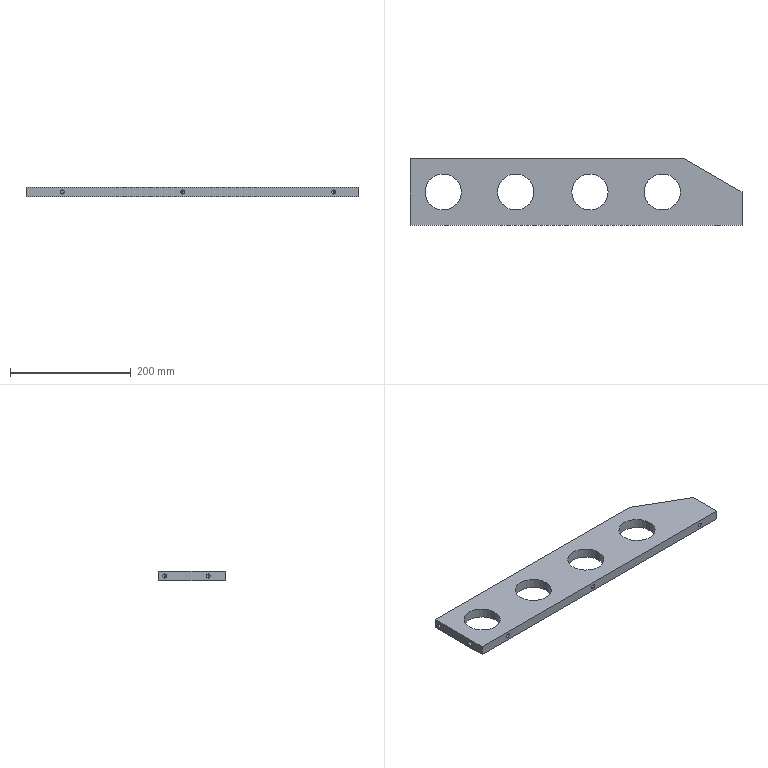Part | SolidWorks | features HoleWzd 4, ICE 4, LibraryFeature 2, Chamfer 1, Cut 1, Extrusion 1, Fillet 1 | 1 solid | 34 faces | box 550 x 110 x 16 mm | volume 740256 mm3 | cylinder 18 | cone 9 | plane 7 | commonest cylinder face diameters 6.75 x10 60 x8
STEP:
#1=CARTESIAN_POINT('',(-130.,0.,-8.));
#2=VERTEX_POINT('',#1);
#3=CARTESIAN_POINT('',(-70.,0.,-8.));
#4=VERTEX_POINT('',#3);
#5=CARTESIAN_POINT('',(-100.,0.,-8.));
#6=DIRECTION('',(0.,0.,1.));
#7=DIRECTION('',(1.,0.,0.));
#8=AXIS2_PLACEMENT_3D('',#5,#6,#7);
#9=CIRCLE('',#8,30.);
#10=EDGE_CURVE('',#2,#4,#9,.T.);
#11=ORIENTED_EDGE('',*,*,#10,.F.);
#12=CARTESIAN_POINT('',(-130.,0.,8.));
#13=VERTEX_POINT('',#12);
#14=CARTESIAN_POINT('',(-130.,0.,-8.));
#15=DIRECTION('',(0.,0.,1.));
#16=VECTOR('',#15,1000.);
#17=LINE('',#14,#16);
#18=EDGE_CURVE('',#2,#13,#17,.T.);
#19=ORIENTED_EDGE('',*,*,#18,.T.);
#20=CARTESIAN_POINT('',(-70.,0.,8.));
#21=VERTEX_POINT('',#20);
#22=CARTESIAN_POINT('',(-100.,0.,8.));
#23=DIRECTION('',(0.,0.,1.));
#24=DIRECTION('',(1.,0.,0.));
#25=AXIS2_PLACEMENT_3D('',#22,#23,#24);
#26=CIRCLE('',#25,30.);
#27=EDGE_CURVE('',#13,#21,#26,.T.);
#28=ORIENTED_EDGE('',*,*,#27,.T.);
#29=CARTESIAN_POINT('',(-70.,0.,-8.));
#30=DIRECTION('',(0.,0.,1.));
#31=VECTOR('',#30,1000.);
#32=LINE('',#29,#31);
#33=EDGE_CURVE('',#4,#21,#32,.T.);
#34=ORIENTED_EDGE('',*,*,#33,.F.);
#35=EDGE_LOOP('',(#11,#19,#28,#34));
#36=FACE_OUTER_BOUND('',#35,.T.);
#37=CARTESIAN_POINT('',(-100.,0.,-8.));
#38=DIRECTION('',(0.,0.,1.));
#39=DIRECTION('',(1.,0.,0.));
#40=AXIS2_PLACEMENT_3D('',#37,#38,#39);
#41=CYLINDRICAL_SURFACE('',#40,30.);
#42=ADVANCED_FACE('',(#36),#41,.F.);
#43=CARTESIAN_POINT('',(-6.962,0.,-8.));
#44=VERTEX_POINT('',#43);
#45=CARTESIAN_POINT('',(53.038,0.,-8.));
#46=VERTEX_POINT('',#45);
#47=CARTESIAN_POINT('',(23.038,0.,-8.));
#48=DIRECTION('',(0.,0.,1.));
#49=DIRECTION('',(-1.,0.,0.));
#50=AXIS2_PLACEMENT_3D('',#47,#48,#49);
#51=CIRCLE('',#50,30.);
#52=EDGE_CURVE('',#44,#46,#51,.T.);
#53=ORIENTED_EDGE('',*,*,#52,.F.);
#54=CARTESIAN_POINT('',(-6.962,0.,8.));
#55=VERTEX_POINT('',#54);
#56=CARTESIAN_POINT('',(-6.962,0.,-8.));
#57=DIRECTION('',(0.,0.,1.));
#58=VECTOR('',#57,1000.);
#59=LINE('',#56,#58);
#60=EDGE_CURVE('',#44,#55,#59,.T.);
#61=ORIENTED_EDGE('',*,*,#60,.T.);
#62=CARTESIAN_POINT('',(53.038,0.,8.));
#63=VERTEX_POINT('',#62);
#64=CARTESIAN_POINT('',(23.038,0.,8.));
#65=DIRECTION('',(0.,0.,1.));
#66=DIRECTION('',(-1.,0.,0.));
#67=AXIS2_PLACEMENT_3D('',#64,#65,#66);
#68=CIRCLE('',#67,30.);
#69=EDGE_CURVE('',#55,#63,#68,.T.);
#70=ORIENTED_EDGE('',*,*,#69,.T.);
#71=CARTESIAN_POINT('',(53.038,0.,-8.));
#72=DIRECTION('',(0.,0.,1.));
#73=VECTOR('',#72,1000.);
#74=LINE('',#71,#73);
#75=EDGE_CURVE('',#46,#63,#74,.T.);
#76=ORIENTED_EDGE('',*,*,#75,.F.);
#77=EDGE_LOOP('',(#53,#61,#70,#76));
#78=FACE_OUTER_BOUND('',#77,.T.);
#79=CARTESIAN_POINT('',(23.038,0.,-8.));
#80=DIRECTION('',(0.,0.,1.));
#81=DIRECTION('',(1.,0.,0.));
#82=AXIS2_PLACEMENT_3D('',#79,#80,#81);
#83=CYLINDRICAL_SURFACE('',#82,30.);
#84=ADVANCED_FACE('',(#78),#83,.F.);
#85=CARTESIAN_POINT('',(113.038,0.,-8.));
#86=VERTEX_POINT('',#85);
#87=CARTESIAN_POINT('',(173.038,0.,-8.));
#88=VERTEX_POINT('',#87);
#89=CARTESIAN_POINT('',(143.038,0.,-8.));
#90=DIRECTION('',(0.,0.,1.));
#91=DIRECTION('',(-1.,0.,0.));
#92=AXIS2_PLACEMENT_3D('',#89,#90,#91);
#93=CIRCLE('',#92,30.);
#94=EDGE_CURVE('',#86,#88,#93,.T.);
#95=ORIENTED_EDGE('',*,*,#94,.F.);
#96=CARTESIAN_POINT('',(113.038,0.,8.));
#97=VERTEX_POINT('',#96);
#98=CARTESIAN_POINT('',(113.038,0.,-8.));
#99=DIRECTION('',(0.,0.,1.));
#100=VECTOR('',#99,1000.);
#101=LINE('',#98,#100);
#102=EDGE_CURVE('',#86,#97,#101,.T.);
#103=ORIENTED_EDGE('',*,*,#102,.T.);
#104=CARTESIAN_POINT('',(173.038,0.,8.));
#105=VERTEX_POINT('',#104);
#106=CARTESIAN_POINT('',(143.038,0.,8.));
#107=DIRECTION('',(0.,0.,1.));
#108=DIRECTION('',(-1.,0.,0.));
#109=AXIS2_PLACEMENT_3D('',#106,#107,#108);
#110=CIRCLE('',#109,30.);
#111=EDGE_CURVE('',#97,#105,#110,.T.);
#112=ORIENTED_EDGE('',*,*,#111,.T.);
#113=CARTESIAN_POINT('',(173.038,0.,-8.));
#114=DIRECTION('',(0.,0.,1.));
#115=VECTOR('',#114,1000.);
#116=LINE('',#113,#115);
#117=EDGE_CURVE('',#88,#105,#116,.T.);
#118=ORIENTED_EDGE('',*,*,#117,.F.);
#119=EDGE_LOOP('',(#95,#103,#112,#118));
#120=FACE_OUTER_BOUND('',#119,.T.);
#121=CARTESIAN_POINT('',(143.038,0.,-8.));
#122=DIRECTION('',(0.,0.,1.));
#123=DIRECTION('',(1.,0.,0.));
#124=AXIS2_PLACEMENT_3D('',#121,#122,#123);
#125=CYLINDRICAL_SURFACE('',#124,30.);
#126=ADVANCED_FACE('',(#120),#125,.F.);
#127=CARTESIAN_POINT('',(-212.319,-29.,2.05));
#128=VERTEX_POINT('',#127);
#129=CARTESIAN_POINT('',(-212.319,-29.,-2.05));
#130=VERTEX_POINT('',#129);
#131=CARTESIAN_POINT('',(-212.319,-29.,2.05));
#132=CARTESIAN_POINT('',(-212.241,-28.979,1.891));
#133=CARTESIAN_POINT('',(-212.171,-28.961,1.727));
#134=CARTESIAN_POINT('',(-212.053,-28.928,1.395));
#135=CARTESIAN_POINT('',(-212.003,-28.915,1.226));
#136=CARTESIAN_POINT('',(-211.883,-28.881,0.711));
#137=CARTESIAN_POINT('',(-211.842,-28.869,0.352));
#138=CARTESIAN_POINT('',(-211.842,-28.87,-0.3557));
#139=CARTESIAN_POINT('',(-211.882,-28.881,-0.7066));
#140=CARTESIAN_POINT('',(-212.045,-28.926,-1.403));
#141=CARTESIAN_POINT('',(-212.164,-28.959,-1.734));
#142=CARTESIAN_POINT('',(-212.319,-29.,-2.05));
#143=B_SPLINE_CURVE_WITH_KNOTS('',3,(#131,#132,#133,#134,#135,#136,#137,#138,#139,#140,#141,#142),.UNSPECIFIED.,.F.,.F.,(4,2,2,2,2,4),(0.001429,0.001958,0.002488,0.003547,0.004606,0.005665),.UNSPECIFIED.);
#144=EDGE_CURVE('',#128,#130,#143,.T.);
#145=ORIENTED_EDGE('',*,*,#144,.F.);
#146=CARTESIAN_POINT('',(-215.,-29.58,3.375));
#147=VERTEX_POINT('',#146);
#148=CARTESIAN_POINT('',(-215.,-29.58,3.375));
#149=CARTESIAN_POINT('',(-214.739,-29.536,3.375));
#150=CARTESIAN_POINT('',(-214.483,-29.489,3.345));
#151=CARTESIAN_POINT('',(-213.983,-29.391,3.228));
#152=CARTESIAN_POINT('',(-213.736,-29.34,3.14));
#153=CARTESIAN_POINT('',(-213.276,-29.238,2.913));
#154=CARTESIAN_POINT('',(-213.06,-29.187,2.774));
#155=CARTESIAN_POINT('',(-212.658,-29.088,2.444));
#156=CARTESIAN_POINT('',(-212.478,-29.042,2.258));
#157=CARTESIAN_POINT('',(-212.319,-29.,2.05));
#158=B_SPLINE_CURVE_WITH_KNOTS('',3,(#148,#149,#150,#151,#152,#153,#154,#155,#156,#157),.UNSPECIFIED.,.F.,.F.,(4,2,2,2,4),(0.01373,0.01451,0.01529,0.01608,0.01686),.UNSPECIFIED.);
#159=EDGE_CURVE('',#147,#128,#158,.T.);
#160=ORIENTED_EDGE('',*,*,#159,.F.);
#161=CARTESIAN_POINT('',(-215.,-29.58,-3.375));
#162=VERTEX_POINT('',#161);
#163=CARTESIAN_POINT('',(-215.,-29.58,-3.375));
#164=CARTESIAN_POINT('',(-215.218,-29.617,-3.375));
#165=CARTESIAN_POINT('',(-215.44,-29.652,-3.353));
#166=CARTESIAN_POINT('',(-215.87,-29.715,-3.268));
#167=CARTESIAN_POINT('',(-216.079,-29.743,-3.205));
#168=CARTESIAN_POINT('',(-216.487,-29.794,-3.038));
#169=CARTESIAN_POINT('',(-216.685,-29.817,-2.933));
#170=CARTESIAN_POINT('',(-217.051,-29.855,-2.689));
#171=CARTESIAN_POINT('',(-217.222,-29.872,-2.55));
#172=CARTESIAN_POINT('',(-217.538,-29.899,-2.236));
#173=CARTESIAN_POINT('',(-217.679,-29.91,-2.064));
#174=CARTESIAN_POINT('',(-217.925,-29.928,-1.698));
#175=CARTESIAN_POINT('',(-218.031,-29.935,-1.501));
#176=CARTESIAN_POINT('',(-218.202,-29.946,-1.09));
#177=CARTESIAN_POINT('',(-218.266,-29.95,-0.8789));
#178=CARTESIAN_POINT('',(-218.353,-29.955,-0.4449));
#179=CARTESIAN_POINT('',(-218.375,-29.956,-0.2203));
#180=CARTESIAN_POINT('',(-218.375,-29.956,0.2219));
#181=CARTESIAN_POINT('',(-218.353,-29.955,0.4417));
#182=CARTESIAN_POINT('',(-218.266,-29.95,0.8784));
#183=CARTESIAN_POINT('',(-218.201,-29.946,1.092));
#184=CARTESIAN_POINT('',(-218.031,-29.935,1.5));
#185=CARTESIAN_POINT('',(-217.926,-29.928,1.696));
#186=CARTESIAN_POINT('',(-217.678,-29.91,2.066));
#187=CARTESIAN_POINT('',(-217.537,-29.899,2.236));
#188=CARTESIAN_POINT('',(-217.225,-29.872,2.548));
#189=CARTESIAN_POINT('',(-217.05,-29.855,2.69));
#190=CARTESIAN_POINT('',(-216.683,-29.817,2.934));
#191=CARTESIAN_POINT('',(-216.489,-29.795,3.037));
#192=CARTESIAN_POINT('',(-216.081,-29.744,3.205));
#193=CARTESIAN_POINT('',(-215.867,-29.715,3.269));
#194=CARTESIAN_POINT('',(-215.438,-29.652,3.354));
#195=CARTESIAN_POINT('',(-215.221,-29.618,3.375));
#196=CARTESIAN_POINT('',(-215.,-29.58,3.375));
#197=B_SPLINE_CURVE_WITH_KNOTS('',3,(#163,#164,#165,#166,#167,#168,#169,#170,#171,#172,#173,#174,#175,#176,#177,#178,#179,#180,#181,#182,#183,#184,#185,#186,#187,#188,#189,#190,#191,#192,#193,#194,#195,#196),.UNSPECIFIED.,.F.,.F.,(4,2,2,2,2,2,2,2,2,2,2,2,2,2,2,2,4),(0.003138,0.0038,0.004462,0.005124,0.005786,0.006447,0.007109,0.007771,0.008433,0.009095,0.009756,0.01042,0.01108,0.01174,0.0124,0.01307,0.01373),.UNSPECIFIED.);
#198=EDGE_CURVE('',#162,#147,#197,.T.);
#199=ORIENTED_EDGE('',*,*,#198,.F.);
#200=CARTESIAN_POINT('',(-212.319,-29.,-2.05));
#201=CARTESIAN_POINT('',(-212.478,-29.042,-2.258));
#202=CARTESIAN_POINT('',(-212.657,-29.088,-2.443));
#203=CARTESIAN_POINT('',(-213.055,-29.186,-2.77));
#204=CARTESIAN_POINT('',(-213.276,-29.238,-2.913));
#205=CARTESIAN_POINT('',(-213.736,-29.34,-3.14));
#206=CARTESIAN_POINT('',(-213.979,-29.391,-3.227));
#207=CARTESIAN_POINT('',(-214.486,-29.49,-3.346));
#208=CARTESIAN_POINT('',(-214.742,-29.537,-3.375));
#209=CARTESIAN_POINT('',(-215.,-29.58,-3.375));
#210=B_SPLINE_CURVE_WITH_KNOTS('',3,(#200,#201,#202,#203,#204,#205,#206,#207,#208,#209),.UNSPECIFIED.,.F.,.F.,(4,2,2,2,4),(0.,0.0007846,0.001569,0.002354,0.003138),.UNSPECIFIED.);
#211=EDGE_CURVE('',#130,#162,#210,.T.);
#212=ORIENTED_EDGE('',*,*,#211,.F.);
#213=EDGE_LOOP('',(#145,#160,#199,#212));
#214=FACE_BOUND('',#213,.T.);
#215=CARTESIAN_POINT('',(-250.,0.,-8.));
#216=VERTEX_POINT('',#215);
#217=CARTESIAN_POINT('',(-190.,0.,-8.));
#218=VERTEX_POINT('',#217);
#219=CARTESIAN_POINT('',(-220.,0.,-8.));
#220=DIRECTION('',(0.,0.,1.));
#221=DIRECTION('',(1.,0.,0.));
#222=AXIS2_PLACEMENT_3D('',#219,#220,#221);
#223=CIRCLE('',#222,30.);
#224=EDGE_CURVE('',#216,#218,#223,.T.);
#225=ORIENTED_EDGE('',*,*,#224,.F.);
#226=CARTESIAN_POINT('',(-250.,0.,8.));
#227=VERTEX_POINT('',#226);
#228=CARTESIAN_POINT('',(-250.,0.,-8.));
#229=DIRECTION('',(0.,0.,1.));
#230=VECTOR('',#229,1000.);
#231=LINE('',#228,#230);
#232=EDGE_CURVE('',#216,#227,#231,.T.);
#233=ORIENTED_EDGE('',*,*,#232,.T.);
#234=CARTESIAN_POINT('',(-190.,0.,8.));
#235=VERTEX_POINT('',#234);
#236=CARTESIAN_POINT('',(-220.,0.,8.));
#237=DIRECTION('',(0.,0.,1.));
#238=DIRECTION('',(1.,0.,0.));
#239=AXIS2_PLACEMENT_3D('',#236,#237,#238);
#240=CIRCLE('',#239,30.);
#241=EDGE_CURVE('',#227,#235,#240,.T.);
#242=ORIENTED_EDGE('',*,*,#241,.T.);
#243=CARTESIAN_POINT('',(-190.,0.,-8.));
#244=DIRECTION('',(0.,0.,1.));
#245=VECTOR('',#244,1000.);
#246=LINE('',#243,#245);
#247=EDGE_CURVE('',#218,#235,#246,.T.);
#248=ORIENTED_EDGE('',*,*,#247,.F.);
#249=EDGE_LOOP('',(#225,#233,#242,#248));
#250=FACE_OUTER_BOUND('',#249,.T.);
#251=CARTESIAN_POINT('',(-220.,0.,-8.));
#252=DIRECTION('',(0.,0.,1.));
#253=DIRECTION('',(1.,0.,0.));
#254=AXIS2_PLACEMENT_3D('',#251,#252,#253);
#255=CYLINDRICAL_SURFACE('',#254,30.);
#256=ADVANCED_FACE('',(#214,#250),#255,.F.);
#257=CARTESIAN_POINT('',(-244.972,-27.,0.));
#258=VERTEX_POINT('',#257);
#259=CARTESIAN_POINT('',(-247.,-27.,3.375));
#260=VERTEX_POINT('',#259);
#261=CARTESIAN_POINT('',(-247.,-27.,3.375));
#262=DIRECTION('',(-0.515,0.,0.8572));
#263=VECTOR('',#262,1000.);
#264=LINE('',#261,#263);
#265=EDGE_CURVE('',#258,#260,#264,.T.);
#266=ORIENTED_EDGE('',*,*,#265,.F.);
#267=CARTESIAN_POINT('',(-247.,-27.,-3.375));
#268=VERTEX_POINT('',#267);
#269=CARTESIAN_POINT('',(-247.,-27.,-3.375));
#270=DIRECTION('',(-0.515,0.,-0.8572));
#271=VECTOR('',#270,1000.);
#272=LINE('',#269,#271);
#273=EDGE_CURVE('',#258,#268,#272,.T.);
#274=ORIENTED_EDGE('',*,*,#273,.T.);
#275=CARTESIAN_POINT('',(-247.,-27.,0.));
#276=DIRECTION('',(-1.,0.,0.));
#277=DIRECTION('',(0.,0.,1.));
#278=AXIS2_PLACEMENT_3D('',#275,#276,#277);
#279=CIRCLE('',#278,3.375);
#280=EDGE_CURVE('',#268,#260,#279,.T.);
#281=ORIENTED_EDGE('',*,*,#280,.T.);
#282=EDGE_LOOP('',(#266,#274,#281));
#283=FACE_OUTER_BOUND('',#282,.T.);
#284=CARTESIAN_POINT('',(-247.,-27.,0.));
#285=DIRECTION('',(-1.,0.,0.));
#286=DIRECTION('',(0.,0.,1.));
#287=AXIS2_PLACEMENT_3D('',#284,#285,#286);
#288=CONICAL_SURFACE('',#287,3.375,1.03);
#289=ADVANCED_FACE('',(#283),#288,.F.);
#290=ORIENTED_EDGE('',*,*,#280,.F.);
#291=CARTESIAN_POINT('',(-275.,-27.,-3.375));
#292=VERTEX_POINT('',#291);
#293=CARTESIAN_POINT('',(-275.,-27.,-3.375));
#294=DIRECTION('',(-1.,0.,0.));
#295=VECTOR('',#294,1000.);
#296=LINE('',#293,#295);
#297=EDGE_CURVE('',#268,#292,#296,.T.);
#298=ORIENTED_EDGE('',*,*,#297,.T.);
#299=CARTESIAN_POINT('',(-275.,-27.,3.375));
#300=VERTEX_POINT('',#299);
#301=CARTESIAN_POINT('',(-275.,-27.,0.));
#302=DIRECTION('',(-1.,0.,0.));
#303=DIRECTION('',(0.,0.,1.));
#304=AXIS2_PLACEMENT_3D('',#301,#302,#303);
#305=CIRCLE('',#304,3.375);
#306=EDGE_CURVE('',#292,#300,#305,.T.);
#307=ORIENTED_EDGE('',*,*,#306,.T.);
#308=CARTESIAN_POINT('',(-275.,-27.,3.375));
#309=DIRECTION('',(-1.,0.,0.));
#310=VECTOR('',#309,1000.);
#311=LINE('',#308,#310);
#312=EDGE_CURVE('',#260,#300,#311,.T.);
#313=ORIENTED_EDGE('',*,*,#312,.F.);
#314=EDGE_LOOP('',(#290,#298,#307,#313));
#315=FACE_OUTER_BOUND('',#314,.T.);
#316=CARTESIAN_POINT('',(-275.,-27.,0.));
#317=DIRECTION('',(-1.,0.,0.));
#318=DIRECTION('',(0.,0.,1.));
#319=AXIS2_PLACEMENT_3D('',#316,#317,#318);
#320=CYLINDRICAL_SURFACE('',#319,3.375);
#321=ADVANCED_FACE('',(#315),#320,.F.);
#322=CARTESIAN_POINT('',(-244.972,45.,0.));
#323=VERTEX_POINT('',#322);
#324=CARTESIAN_POINT('',(-247.,45.,3.375));
#325=VERTEX_POINT('',#324);
#326=CARTESIAN_POINT('',(-247.,45.,3.375));
#327=DIRECTION('',(-0.515,0.,0.8572));
#328=VECTOR('',#327,1000.);
#329=LINE('',#326,#328);
#330=EDGE_CURVE('',#323,#325,#329,.T.);
#331=ORIENTED_EDGE('',*,*,#330,.F.);
#332=CARTESIAN_POINT('',(-247.,45.,-3.375));
#333=VERTEX_POINT('',#332);
#334=CARTESIAN_POINT('',(-247.,45.,-3.375));
#335=DIRECTION('',(-0.515,0.,-0.8572));
#336=VECTOR('',#335,1000.);
#337=LINE('',#334,#336);
#338=EDGE_CURVE('',#323,#333,#337,.T.);
#339=ORIENTED_EDGE('',*,*,#338,.T.);
#340=CARTESIAN_POINT('',(-247.,45.,0.));
#341=DIRECTION('',(-1.,0.,0.));
#342=DIRECTION('',(0.,0.,1.));
#343=AXIS2_PLACEMENT_3D('',#340,#341,#342);
#344=CIRCLE('',#343,3.375);
#345=EDGE_CURVE('',#333,#325,#344,.T.);
#346=ORIENTED_EDGE('',*,*,#345,.T.);
#347=EDGE_LOOP('',(#331,#339,#346));
#348=FACE_OUTER_BOUND('',#347,.T.);
#349=CARTESIAN_POINT('',(-247.,45.,0.));
#350=DIRECTION('',(-1.,0.,0.));
#351=DIRECTION('',(0.,0.,1.));
#352=AXIS2_PLACEMENT_3D('',#349,#350,#351);
#353=CONICAL_SURFACE('',#352,3.375,1.03);
#354=ADVANCED_FACE('',(#348),#353,.F.);
#355=ORIENTED_EDGE('',*,*,#345,.F.);
#356=CARTESIAN_POINT('',(-275.,45.,-3.375));
#357=VERTEX_POINT('',#356);
#358=CARTESIAN_POINT('',(-275.,45.,-3.375));
#359=DIRECTION('',(-1.,0.,0.));
#360=VECTOR('',#359,1000.);
#361=LINE('',#358,#360);
#362=EDGE_CURVE('',#333,#357,#361,.T.);
#363=ORIENTED_EDGE('',*,*,#362,.T.);
#364=CARTESIAN_POINT('',(-275.,45.,3.375));
#365=VERTEX_POINT('',#364);
#366=CARTESIAN_POINT('',(-275.,45.,0.));
#367=DIRECTION('',(-1.,0.,0.));
#368=DIRECTION('',(0.,0.,1.));
#369=AXIS2_PLACEMENT_3D('',#366,#367,#368);
#370=CIRCLE('',#369,3.375);
#371=EDGE_CURVE('',#357,#365,#370,.T.);
#372=ORIENTED_EDGE('',*,*,#371,.T.);
#373=CARTESIAN_POINT('',(-275.,45.,3.375));
#374=DIRECTION('',(-1.,0.,0.));
#375=VECTOR('',#374,1000.);
#376=LINE('',#373,#375);
#377=EDGE_CURVE('',#325,#365,#376,.T.);
#378=ORIENTED_EDGE('',*,*,#377,.F.);
#379=EDGE_LOOP('',(#355,#363,#372,#378));
#380=FACE_OUTER_BOUND('',#379,.T.);
#381=CARTESIAN_POINT('',(-275.,45.,0.));
#382=DIRECTION('',(-1.,0.,0.));
#383=DIRECTION('',(0.,0.,1.));
#384=AXIS2_PLACEMENT_3D('',#381,#382,#383);
#385=CYLINDRICAL_SURFACE('',#384,3.375);
#386=ADVANCED_FACE('',(#380),#385,.F.);
#387=ORIENTED_EDGE('',*,*,#198,.T.);
#388=CARTESIAN_POINT('',(-215.,-55.,3.375));
#389=VERTEX_POINT('',#388);
#390=CARTESIAN_POINT('',(-215.,-55.,3.375));
#391=DIRECTION('',(0.,-1.,0.));
#392=VECTOR('',#391,1000.);
#393=LINE('',#390,#392);
#394=EDGE_CURVE('',#147,#389,#393,.T.);
#395=ORIENTED_EDGE('',*,*,#394,.T.);
#396=CARTESIAN_POINT('',(-215.,-55.,-3.375));
#397=VERTEX_POINT('',#396);
#398=CARTESIAN_POINT('',(-215.,-55.,0.));
#399=DIRECTION('',(0.,-1.,0.));
#400=DIRECTION('',(0.,0.,-1.));
#401=AXIS2_PLACEMENT_3D('',#398,#399,#400);
#402=CIRCLE('',#401,3.375);
#403=EDGE_CURVE('',#389,#397,#402,.T.);
#404=ORIENTED_EDGE('',*,*,#403,.T.);
#405=CARTESIAN_POINT('',(-215.,-55.,-3.375));
#406=DIRECTION('',(0.,-1.,0.));
#407=VECTOR('',#406,1000.);
#408=LINE('',#405,#407);
#409=EDGE_CURVE('',#162,#397,#408,.T.);
#410=ORIENTED_EDGE('',*,*,#409,.F.);
#411=EDGE_LOOP('',(#387,#395,#404,#410));
#412=FACE_OUTER_BOUND('',#411,.T.);
#413=CARTESIAN_POINT('',(-215.,-55.,0.));
#414=DIRECTION('',(0.,-1.,0.));
#415=DIRECTION('',(0.,0.,-1.));
#416=AXIS2_PLACEMENT_3D('',#413,#414,#415);
#417=CYLINDRICAL_SURFACE('',#416,3.375);
#418=ADVANCED_FACE('',(#412),#417,.F.);
#419=CARTESIAN_POINT('',(-15.,-26.972,0.));
#420=VERTEX_POINT('',#419);
#421=CARTESIAN_POINT('',(-15.,-29.,-3.375));
#422=VERTEX_POINT('',#421);
#423=CARTESIAN_POINT('',(-15.,-29.,-3.375));
#424=DIRECTION('',(0.,-0.515,-0.8572));
#425=VECTOR('',#424,1000.);
#426=LINE('',#423,#425);
#427=EDGE_CURVE('',#420,#422,#426,.T.);
#428=ORIENTED_EDGE('',*,*,#427,.F.);
#429=CARTESIAN_POINT('',(-15.,-29.,3.375));
#430=VERTEX_POINT('',#429);
#431=CARTESIAN_POINT('',(-15.,-29.,3.375));
#432=DIRECTION('',(0.,-0.515,0.8572));
#433=VECTOR('',#432,1000.);
#434=LINE('',#431,#433);
#435=EDGE_CURVE('',#420,#430,#434,.T.);
#436=ORIENTED_EDGE('',*,*,#435,.T.);
#437=CARTESIAN_POINT('',(-15.,-29.,0.));
#438=DIRECTION('',(0.,-1.,0.));
#439=DIRECTION('',(0.,0.,-1.));
#440=AXIS2_PLACEMENT_3D('',#437,#438,#439);
#441=CIRCLE('',#440,3.375);
#442=EDGE_CURVE('',#430,#422,#441,.T.);
#443=ORIENTED_EDGE('',*,*,#442,.T.);
#444=EDGE_LOOP('',(#428,#436,#443));
#445=FACE_OUTER_BOUND('',#444,.T.);
#446=CARTESIAN_POINT('',(-15.,-29.,0.));
#447=DIRECTION('',(0.,-1.,0.));
#448=DIRECTION('',(0.,0.,-1.));
#449=AXIS2_PLACEMENT_3D('',#446,#447,#448);
#450=CONICAL_SURFACE('',#449,3.375,1.03);
#451=ADVANCED_FACE('',(#445),#450,.F.);
#452=ORIENTED_EDGE('',*,*,#442,.F.);
#453=CARTESIAN_POINT('',(-15.,-55.,3.375));
#454=VERTEX_POINT('',#453);
#455=CARTESIAN_POINT('',(-15.,-55.,3.375));
#456=DIRECTION('',(0.,-1.,0.));
#457=VECTOR('',#456,1000.);
#458=LINE('',#455,#457);
#459=EDGE_CURVE('',#430,#454,#458,.T.);
#460=ORIENTED_EDGE('',*,*,#459,.T.);
#461=CARTESIAN_POINT('',(-15.,-55.,-3.375));
#462=VERTEX_POINT('',#461);
#463=CARTESIAN_POINT('',(-15.,-55.,0.));
#464=DIRECTION('',(0.,-1.,0.));
#465=DIRECTION('',(0.,0.,-1.));
#466=AXIS2_PLACEMENT_3D('',#463,#464,#465);
#467=CIRCLE('',#466,3.375);
#468=EDGE_CURVE('',#454,#462,#467,.T.);
#469=ORIENTED_EDGE('',*,*,#468,.T.);
#470=CARTESIAN_POINT('',(-15.,-55.,-3.375));
#471=DIRECTION('',(0.,-1.,0.));
#472=VECTOR('',#471,1000.);
#473=LINE('',#470,#472);
#474=EDGE_CURVE('',#422,#462,#473,.T.);
#475=ORIENTED_EDGE('',*,*,#474,.F.);
#476=EDGE_LOOP('',(#452,#460,#469,#475));
#477=FACE_OUTER_BOUND('',#476,.T.);
#478=CARTESIAN_POINT('',(-15.,-55.,0.));
#479=DIRECTION('',(0.,-1.,0.));
#480=DIRECTION('',(0.,0.,-1.));
#481=AXIS2_PLACEMENT_3D('',#478,#479,#480);
#482=CYLINDRICAL_SURFACE('',#481,3.375);
#483=ADVANCED_FACE('',(#477),#482,.F.);
#484=CARTESIAN_POINT('',(235.,-26.972,0.));
#485=VERTEX_POINT('',#484);
#486=CARTESIAN_POINT('',(235.,-29.,-3.375));
#487=VERTEX_POINT('',#486);
#488=CARTESIAN_POINT('',(235.,-29.,-3.375));
#489=DIRECTION('',(0.,-0.515,-0.8572));
#490=VECTOR('',#489,1000.);
#491=LINE('',#488,#490);
#492=EDGE_CURVE('',#485,#487,#491,.T.);
#493=ORIENTED_EDGE('',*,*,#492,.F.);
#494=CARTESIAN_POINT('',(235.,-29.,3.375));
#495=VERTEX_POINT('',#494);
#496=CARTESIAN_POINT('',(235.,-29.,3.375));
#497=DIRECTION('',(0.,-0.515,0.8572));
#498=VECTOR('',#497,1000.);
#499=LINE('',#496,#498);
#500=EDGE_CURVE('',#485,#495,#499,.T.);
#501=ORIENTED_EDGE('',*,*,#500,.T.);
#502=CARTESIAN_POINT('',(235.,-29.,0.));
#503=DIRECTION('',(0.,-1.,0.));
#504=DIRECTION('',(0.,0.,-1.));
#505=AXIS2_PLACEMENT_3D('',#502,#503,#504);
#506=CIRCLE('',#505,3.375);
#507=EDGE_CURVE('',#495,#487,#506,.T.);
#508=ORIENTED_EDGE('',*,*,#507,.T.);
#509=EDGE_LOOP('',(#493,#501,#508));
#510=FACE_OUTER_BOUND('',#509,.T.);
#511=CARTESIAN_POINT('',(235.,-29.,0.));
#512=DIRECTION('',(0.,-1.,0.));
#513=DIRECTION('',(0.,0.,-1.));
#514=AXIS2_PLACEMENT_3D('',#511,#512,#513);
#515=CONICAL_SURFACE('',#514,3.375,1.03);
#516=ADVANCED_FACE('',(#510),#515,.F.);
#517=ORIENTED_EDGE('',*,*,#507,.F.);
#518=CARTESIAN_POINT('',(235.,-55.,3.375));
#519=VERTEX_POINT('',#518);
#520=CARTESIAN_POINT('',(235.,-55.,3.375));
#521=DIRECTION('',(0.,-1.,0.));
#522=VECTOR('',#521,1000.);
#523=LINE('',#520,#522);
#524=EDGE_CURVE('',#495,#519,#523,.T.);
#525=ORIENTED_EDGE('',*,*,#524,.T.);
#526=CARTESIAN_POINT('',(235.,-55.,-3.375));
#527=VERTEX_POINT('',#526);
#528=CARTESIAN_POINT('',(235.,-55.,0.));
#529=DIRECTION('',(0.,-1.,0.));
#530=DIRECTION('',(0.,0.,-1.));
#531=AXIS2_PLACEMENT_3D('',#528,#529,#530);
#532=CIRCLE('',#531,3.375);
#533=EDGE_CURVE('',#519,#527,#532,.T.);
#534=ORIENTED_EDGE('',*,*,#533,.T.);
#535=CARTESIAN_POINT('',(235.,-55.,-3.375));
#536=DIRECTION('',(0.,-1.,0.));
#537=VECTOR('',#536,1000.);
#538=LINE('',#535,#537);
#539=EDGE_CURVE('',#487,#527,#538,.T.);
#540=ORIENTED_EDGE('',*,*,#539,.F.);
#541=EDGE_LOOP('',(#517,#525,#534,#540));
#542=FACE_OUTER_BOUND('',#541,.T.);
#543=CARTESIAN_POINT('',(235.,-55.,0.));
#544=DIRECTION('',(0.,-1.,0.));
#545=DIRECTION('',(0.,0.,-1.));
#546=AXIS2_PLACEMENT_3D('',#543,#544,#545);
#547=CYLINDRICAL_SURFACE('',#546,3.375);
#548=ADVANCED_FACE('',(#542),#547,.F.);
#549=CARTESIAN_POINT('',(275.,0.,8.));
#550=VERTEX_POINT('',#549);
#551=CARTESIAN_POINT('',(275.,0.,-8.));
#552=VERTEX_POINT('',#551);
#553=CARTESIAN_POINT('',(275.,0.,729.4));
#554=DIRECTION('',(0.,0.,-1.));
#555=VECTOR('',#554,1000.);
#556=LINE('',#553,#555);
#557=EDGE_CURVE('',#550,#552,#556,.T.);
#558=ORIENTED_EDGE('',*,*,#557,.F.);
#559=CARTESIAN_POINT('',(275.,-55.,8.));
#560=VERTEX_POINT('',#559);
#561=CARTESIAN_POINT('',(275.,-55.,8.));
#562=DIRECTION('',(0.,1.,0.));
#563=VECTOR('',#562,1000.);
#564=LINE('',#561,#563);
#565=EDGE_CURVE('',#560,#550,#564,.T.);
#566=ORIENTED_EDGE('',*,*,#565,.F.);
#567=CARTESIAN_POINT('',(275.,-55.,-8.));
#568=VERTEX_POINT('',#567);
#569=CARTESIAN_POINT('',(275.,-55.,8.));
#570=DIRECTION('',(0.,0.,-1.));
#571=VECTOR('',#570,1000.);
#572=LINE('',#569,#571);
#573=EDGE_CURVE('',#560,#568,#572,.T.);
#574=ORIENTED_EDGE('',*,*,#573,.T.);
#575=CARTESIAN_POINT('',(275.,-55.,-8.));
#576=DIRECTION('',(0.,1.,0.));
#577=VECTOR('',#576,1000.);
#578=LINE('',#575,#577);
#579=EDGE_CURVE('',#568,#552,#578,.T.);
#580=ORIENTED_EDGE('',*,*,#579,.T.);
#581=EDGE_LOOP('',(#558,#566,#574,#580));
#582=FACE_OUTER_BOUND('',#581,.T.);
#583=CARTESIAN_POINT('',(275.,-55.,8.));
#584=DIRECTION('',(-1.,0.,0.));
#585=DIRECTION('',(0.,0.,1.));
#586=AXIS2_PLACEMENT_3D('',#583,#584,#585);
#587=PLANE('',#586);
#588=ADVANCED_FACE('',(#582),#587,.F.);
#589=CARTESIAN_POINT('',(179.737,55.,8.));
#590=VERTEX_POINT('',#589);
#591=CARTESIAN_POINT('',(179.737,55.,-8.));
#592=VERTEX_POINT('',#591);
#593=CARTESIAN_POINT('',(179.737,55.,729.4));
#594=DIRECTION('',(0.,0.,-1.));
#595=VECTOR('',#594,1000.);
#596=LINE('',#593,#595);
#597=EDGE_CURVE('',#590,#592,#596,.T.);
#598=ORIENTED_EDGE('',*,*,#597,.T.);
#599=CARTESIAN_POINT('',(-275.,55.,-8.));
#600=VERTEX_POINT('',#599);
#601=CARTESIAN_POINT('',(-275.,55.,-8.));
#602=DIRECTION('',(-1.,0.,0.));
#603=VECTOR('',#602,1000.);
#604=LINE('',#601,#603);
#605=EDGE_CURVE('',#592,#600,#604,.T.);
#606=ORIENTED_EDGE('',*,*,#605,.T.);
#607=CARTESIAN_POINT('',(-275.,55.,8.));
#608=VERTEX_POINT('',#607);
#609=CARTESIAN_POINT('',(-275.,55.,8.));
#610=DIRECTION('',(0.,0.,-1.));
#611=VECTOR('',#610,1000.);
#612=LINE('',#609,#611);
#613=EDGE_CURVE('',#608,#600,#612,.T.);
#614=ORIENTED_EDGE('',*,*,#613,.F.);
#615=CARTESIAN_POINT('',(-275.,55.,8.));
#616=DIRECTION('',(-1.,0.,0.));
#617=VECTOR('',#616,1000.);
#618=LINE('',#615,#617);
#619=EDGE_CURVE('',#590,#608,#618,.T.);
#620=ORIENTED_EDGE('',*,*,#619,.F.);
#621=EDGE_LOOP('',(#598,#606,#614,#620));
#622=FACE_OUTER_BOUND('',#621,.T.);
#623=CARTESIAN_POINT('',(-275.,55.,8.));
#624=DIRECTION('',(0.,-1.,0.));
#625=DIRECTION('',(0.,0.,-1.));
#626=AXIS2_PLACEMENT_3D('',#623,#624,#625);
#627=PLANE('',#626);
#628=ADVANCED_FACE('',(#622),#627,.F.);
#629=CARTESIAN_POINT('',(-100.,0.,8.));
#630=DIRECTION('',(0.,0.,1.));
#631=DIRECTION('',(1.,0.,0.));
#632=AXIS2_PLACEMENT_3D('',#629,#630,#631);
#633=CIRCLE('',#632,30.);
#634=EDGE_CURVE('',#21,#13,#633,.T.);
#635=ORIENTED_EDGE('',*,*,#634,.F.);
#636=ORIENTED_EDGE('',*,*,#27,.F.);
#637=EDGE_LOOP('',(#635,#636));
#638=FACE_BOUND('',#637,.T.);
#639=CARTESIAN_POINT('',(23.038,0.,8.));
#640=DIRECTION('',(0.,0.,1.));
#641=DIRECTION('',(-1.,0.,0.));
#642=AXIS2_PLACEMENT_3D('',#639,#640,#641);
#643=CIRCLE('',#642,30.);
#644=EDGE_CURVE('',#63,#55,#643,.T.);
#645=ORIENTED_EDGE('',*,*,#644,.F.);
#646=ORIENTED_EDGE('',*,*,#69,.F.);
#647=EDGE_LOOP('',(#645,#646));
#648=FACE_BOUND('',#647,.T.);
#649=CARTESIAN_POINT('',(143.038,0.,8.));
#650=DIRECTION('',(0.,0.,1.));
#651=DIRECTION('',(-1.,0.,0.));
#652=AXIS2_PLACEMENT_3D('',#649,#650,#651);
#653=CIRCLE('',#652,30.);
#654=EDGE_CURVE('',#105,#97,#653,.T.);
#655=ORIENTED_EDGE('',*,*,#654,.F.);
#656=ORIENTED_EDGE('',*,*,#111,.F.);
#657=EDGE_LOOP('',(#655,#656));
#658=FACE_BOUND('',#657,.T.);
#659=CARTESIAN_POINT('',(-220.,0.,8.));
#660=DIRECTION('',(0.,0.,1.));
#661=DIRECTION('',(1.,0.,0.));
#662=AXIS2_PLACEMENT_3D('',#659,#660,#661);
#663=CIRCLE('',#662,30.);
#664=EDGE_CURVE('',#235,#227,#663,.T.);
#665=ORIENTED_EDGE('',*,*,#664,.F.);
#666=ORIENTED_EDGE('',*,*,#241,.F.);
#667=EDGE_LOOP('',(#665,#666));
#668=FACE_BOUND('',#667,.T.);
#669=CARTESIAN_POINT('',(251.184,13.75,8.));
#670=DIRECTION('',(0.866,-0.5,0.));
#671=VECTOR('',#670,1000.);
#672=LINE('',#669,#671);
#673=EDGE_CURVE('',#590,#550,#672,.T.);
#674=ORIENTED_EDGE('',*,*,#673,.F.);
#675=ORIENTED_EDGE('',*,*,#619,.T.);
#676=CARTESIAN_POINT('',(-275.,-55.,8.));
#677=VERTEX_POINT('',#676);
#678=CARTESIAN_POINT('',(-275.,-55.,8.));
#679=DIRECTION('',(0.,-1.,0.));
#680=VECTOR('',#679,1000.);
#681=LINE('',#678,#680);
#682=EDGE_CURVE('',#608,#677,#681,.T.);
#683=ORIENTED_EDGE('',*,*,#682,.T.);
#684=CARTESIAN_POINT('',(-275.,-55.,8.));
#685=DIRECTION('',(1.,0.,0.));
#686=VECTOR('',#685,1000.);
#687=LINE('',#684,#686);
#688=EDGE_CURVE('',#677,#560,#687,.T.);
#689=ORIENTED_EDGE('',*,*,#688,.T.);
#690=ORIENTED_EDGE('',*,*,#565,.T.);
#691=EDGE_LOOP('',(#674,#675,#683,#689,#690));
#692=FACE_OUTER_BOUND('',#691,.T.);
#693=CARTESIAN_POINT('',(275.,55.,8.));
#694=DIRECTION('',(0.,0.,-1.));
#695=DIRECTION('',(-1.,0.,0.));
#696=AXIS2_PLACEMENT_3D('',#693,#694,#695);
#697=PLANE('',#696);
#698=ADVANCED_FACE('',(#638,#648,#658,#668,#692),#697,.F.);
#699=CARTESIAN_POINT('',(-100.,0.,-8.));
#700=DIRECTION('',(0.,0.,1.));
#701=DIRECTION('',(1.,0.,0.));
#702=AXIS2_PLACEMENT_3D('',#699,#700,#701);
#703=CIRCLE('',#702,30.);
#704=EDGE_CURVE('',#4,#2,#703,.T.);
#705=ORIENTED_EDGE('',*,*,#704,.T.);
#706=ORIENTED_EDGE('',*,*,#10,.T.);
#707=EDGE_LOOP('',(#705,#706));
#708=FACE_BOUND('',#707,.T.);
#709=CARTESIAN_POINT('',(23.038,0.,-8.));
#710=DIRECTION('',(0.,0.,1.));
#711=DIRECTION('',(-1.,0.,0.));
#712=AXIS2_PLACEMENT_3D('',#709,#710,#711);
#713=CIRCLE('',#712,30.);
#714=EDGE_CURVE('',#46,#44,#713,.T.);
#715=ORIENTED_EDGE('',*,*,#714,.T.);
#716=ORIENTED_EDGE('',*,*,#52,.T.);
#717=EDGE_LOOP('',(#715,#716));
#718=FACE_BOUND('',#717,.T.);
#719=CARTESIAN_POINT('',(143.038,0.,-8.));
#720=DIRECTION('',(0.,0.,1.));
#721=DIRECTION('',(-1.,0.,0.));
#722=AXIS2_PLACEMENT_3D('',#719,#720,#721);
#723=CIRCLE('',#722,30.);
#724=EDGE_CURVE('',#88,#86,#723,.T.);
#725=ORIENTED_EDGE('',*,*,#724,.T.);
#726=ORIENTED_EDGE('',*,*,#94,.T.);
#727=EDGE_LOOP('',(#725,#726));
#728=FACE_BOUND('',#727,.T.);
#729=CARTESIAN_POINT('',(-220.,0.,-8.));
#730=DIRECTION('',(0.,0.,1.));
#731=DIRECTION('',(1.,0.,0.));
#732=AXIS2_PLACEMENT_3D('',#729,#730,#731);
#733=CIRCLE('',#732,30.);
#734=EDGE_CURVE('',#218,#216,#733,.T.);
#735=ORIENTED_EDGE('',*,*,#734,.T.);
#736=ORIENTED_EDGE('',*,*,#224,.T.);
#737=EDGE_LOOP('',(#735,#736));
#738=FACE_BOUND('',#737,.T.);
#739=ORIENTED_EDGE('',*,*,#605,.F.);
#740=CARTESIAN_POINT('',(251.184,13.75,-8.));
#741=DIRECTION('',(0.866,-0.5,0.));
#742=VECTOR('',#741,1000.);
#743=LINE('',#740,#742);
#744=EDGE_CURVE('',#592,#552,#743,.T.);
#745=ORIENTED_EDGE('',*,*,#744,.T.);
#746=ORIENTED_EDGE('',*,*,#579,.F.);
#747=CARTESIAN_POINT('',(-275.,-55.,-8.));
#748=VERTEX_POINT('',#747);
#749=CARTESIAN_POINT('',(-275.,-55.,-8.));
#750=DIRECTION('',(1.,0.,0.));
#751=VECTOR('',#750,1000.);
#752=LINE('',#749,#751);
#753=EDGE_CURVE('',#748,#568,#752,.T.);
#754=ORIENTED_EDGE('',*,*,#753,.F.);
#755=CARTESIAN_POINT('',(-275.,-55.,-8.));
#756=DIRECTION('',(0.,-1.,0.));
#757=VECTOR('',#756,1000.);
#758=LINE('',#755,#757);
#759=EDGE_CURVE('',#600,#748,#758,.T.);
#760=ORIENTED_EDGE('',*,*,#759,.F.);
#761=EDGE_LOOP('',(#739,#745,#746,#754,#760));
#762=FACE_OUTER_BOUND('',#761,.T.);
#763=CARTESIAN_POINT('',(275.,55.,-8.));
#764=DIRECTION('',(0.,0.,-1.));
#765=DIRECTION('',(-1.,0.,0.));
#766=AXIS2_PLACEMENT_3D('',#763,#764,#765);
#767=PLANE('',#766);
#768=ADVANCED_FACE('',(#708,#718,#728,#738,#762),#767,.T.);
#769=CARTESIAN_POINT('',(-275.,-27.,0.));
#770=DIRECTION('',(-1.,0.,0.));
#771=DIRECTION('',(0.,0.,1.));
#772=AXIS2_PLACEMENT_3D('',#769,#770,#771);
#773=CIRCLE('',#772,3.375);
#774=EDGE_CURVE('',#300,#292,#773,.T.);
#775=ORIENTED_EDGE('',*,*,#774,.F.);
#776=ORIENTED_EDGE('',*,*,#306,.F.);
#777=EDGE_LOOP('',(#775,#776));
#778=FACE_BOUND('',#777,.T.);
#779=CARTESIAN_POINT('',(-275.,45.,0.));
#780=DIRECTION('',(-1.,0.,0.));
#781=DIRECTION('',(0.,0.,1.));
#782=AXIS2_PLACEMENT_3D('',#779,#780,#781);
#783=CIRCLE('',#782,3.375);
#784=EDGE_CURVE('',#365,#357,#783,.T.);
#785=ORIENTED_EDGE('',*,*,#784,.F.);
#786=ORIENTED_EDGE('',*,*,#371,.F.);
#787=EDGE_LOOP('',(#785,#786));
#788=FACE_BOUND('',#787,.T.);
#789=ORIENTED_EDGE('',*,*,#759,.T.);
#790=CARTESIAN_POINT('',(-275.,-55.,8.));
#791=DIRECTION('',(0.,0.,-1.));
#792=VECTOR('',#791,1000.);
#793=LINE('',#790,#792);
#794=EDGE_CURVE('',#677,#748,#793,.T.);
#795=ORIENTED_EDGE('',*,*,#794,.F.);
#796=ORIENTED_EDGE('',*,*,#682,.F.);
#797=ORIENTED_EDGE('',*,*,#613,.T.);
#798=EDGE_LOOP('',(#789,#795,#796,#797));
#799=FACE_OUTER_BOUND('',#798,.T.);
#800=CARTESIAN_POINT('',(-275.,-55.,8.));
#801=DIRECTION('',(1.,0.,0.));
#802=DIRECTION('',(0.,0.,-1.));
#803=AXIS2_PLACEMENT_3D('',#800,#801,#802);
#804=PLANE('',#803);
#805=ADVANCED_FACE('',(#778,#788,#799),#804,.F.);
#806=CARTESIAN_POINT('',(-215.,-55.,0.));
#807=DIRECTION('',(0.,-1.,0.));
#808=DIRECTION('',(0.,0.,-1.));
#809=AXIS2_PLACEMENT_3D('',#806,#807,#808);
#810=CIRCLE('',#809,3.375);
#811=EDGE_CURVE('',#397,#389,#810,.T.);
#812=ORIENTED_EDGE('',*,*,#811,.F.);
#813=ORIENTED_EDGE('',*,*,#403,.F.);
#814=EDGE_LOOP('',(#812,#813));
#815=FACE_BOUND('',#814,.T.);
#816=CARTESIAN_POINT('',(-15.,-55.,0.));
#817=DIRECTION('',(0.,-1.,0.));
#818=DIRECTION('',(0.,0.,-1.));
#819=AXIS2_PLACEMENT_3D('',#816,#817,#818);
#820=CIRCLE('',#819,3.375);
#821=EDGE_CURVE('',#462,#454,#820,.T.);
#822=ORIENTED_EDGE('',*,*,#821,.F.);
#823=ORIENTED_EDGE('',*,*,#468,.F.);
#824=EDGE_LOOP('',(#822,#823));
#825=FACE_BOUND('',#824,.T.);
#826=CARTESIAN_POINT('',(235.,-55.,0.));
#827=DIRECTION('',(0.,-1.,0.));
#828=DIRECTION('',(0.,0.,-1.));
#829=AXIS2_PLACEMENT_3D('',#826,#827,#828);
#830=CIRCLE('',#829,3.375);
#831=EDGE_CURVE('',#527,#519,#830,.T.);
#832=ORIENTED_EDGE('',*,*,#831,.F.);
#833=ORIENTED_EDGE('',*,*,#533,.F.);
#834=EDGE_LOOP('',(#832,#833));
#835=FACE_BOUND('',#834,.T.);
#836=ORIENTED_EDGE('',*,*,#753,.T.);
#837=ORIENTED_EDGE('',*,*,#573,.F.);
#838=ORIENTED_EDGE('',*,*,#688,.F.);
#839=ORIENTED_EDGE('',*,*,#794,.T.);
#840=EDGE_LOOP('',(#836,#837,#838,#839));
#841=FACE_OUTER_BOUND('',#840,.T.);
#842=CARTESIAN_POINT('',(-275.,-55.,8.));
#843=DIRECTION('',(0.,1.,0.));
#844=DIRECTION('',(0.,0.,1.));
#845=AXIS2_PLACEMENT_3D('',#842,#843,#844);
#846=PLANE('',#845);
#847=ADVANCED_FACE('',(#815,#825,#835,#841),#846,.F.);
#848=ORIENTED_EDGE('',*,*,#597,.F.);
#849=ORIENTED_EDGE('',*,*,#673,.T.);
#850=ORIENTED_EDGE('',*,*,#557,.T.);
#851=ORIENTED_EDGE('',*,*,#744,.F.);
#852=EDGE_LOOP('',(#848,#849,#850,#851));
#853=FACE_OUTER_BOUND('',#852,.T.);
#854=CARTESIAN_POINT('',(179.737,55.,729.4));
#855=DIRECTION('',(0.5,0.866,0.));
#856=DIRECTION('',(-0.866,0.5,0.));
#857=AXIS2_PLACEMENT_3D('',#854,#855,#856);
#858=PLANE('',#857);
#859=ADVANCED_FACE('',(#853),#858,.T.);
#860=ORIENTED_EDGE('',*,*,#524,.F.);
#861=CARTESIAN_POINT('',(235.,-29.,0.));
#862=DIRECTION('',(0.,-1.,0.));
#863=DIRECTION('',(0.,0.,-1.));
#864=AXIS2_PLACEMENT_3D('',#861,#862,#863);
#865=CIRCLE('',#864,3.375);
#866=EDGE_CURVE('',#487,#495,#865,.T.);
#867=ORIENTED_EDGE('',*,*,#866,.F.);
#868=ORIENTED_EDGE('',*,*,#539,.T.);
#869=ORIENTED_EDGE('',*,*,#831,.T.);
#870=EDGE_LOOP('',(#860,#867,#868,#869));
#871=FACE_OUTER_BOUND('',#870,.T.);
#872=CARTESIAN_POINT('',(235.,-55.,0.));
#873=DIRECTION('',(0.,-1.,0.));
#874=DIRECTION('',(0.,0.,-1.));
#875=AXIS2_PLACEMENT_3D('',#872,#873,#874);
#876=CYLINDRICAL_SURFACE('',#875,3.375);
#877=ADVANCED_FACE('',(#871),#876,.F.);
#878=ORIENTED_EDGE('',*,*,#500,.F.);
#879=ORIENTED_EDGE('',*,*,#492,.T.);
#880=ORIENTED_EDGE('',*,*,#866,.T.);
#881=EDGE_LOOP('',(#878,#879,#880));
#882=FACE_OUTER_BOUND('',#881,.T.);
#883=CARTESIAN_POINT('',(235.,-29.,0.));
#884=DIRECTION('',(0.,-1.,0.));
#885=DIRECTION('',(0.,0.,-1.));
#886=AXIS2_PLACEMENT_3D('',#883,#884,#885);
#887=CONICAL_SURFACE('',#886,3.375,1.03);
#888=ADVANCED_FACE('',(#882),#887,.F.);
#889=ORIENTED_EDGE('',*,*,#459,.F.);
#890=CARTESIAN_POINT('',(-15.,-29.,0.));
#891=DIRECTION('',(0.,-1.,0.));
#892=DIRECTION('',(0.,0.,-1.));
#893=AXIS2_PLACEMENT_3D('',#890,#891,#892);
#894=CIRCLE('',#893,3.375);
#895=EDGE_CURVE('',#422,#430,#894,.T.);
#896=ORIENTED_EDGE('',*,*,#895,.F.);
#897=ORIENTED_EDGE('',*,*,#474,.T.);
#898=ORIENTED_EDGE('',*,*,#821,.T.);
#899=EDGE_LOOP('',(#889,#896,#897,#898));
#900=FACE_OUTER_BOUND('',#899,.T.);
#901=CARTESIAN_POINT('',(-15.,-55.,0.));
#902=DIRECTION('',(0.,-1.,0.));
#903=DIRECTION('',(0.,0.,-1.));
#904=AXIS2_PLACEMENT_3D('',#901,#902,#903);
#905=CYLINDRICAL_SURFACE('',#904,3.375);
#906=ADVANCED_FACE('',(#900),#905,.F.);
#907=ORIENTED_EDGE('',*,*,#435,.F.);
#908=ORIENTED_EDGE('',*,*,#427,.T.);
#909=ORIENTED_EDGE('',*,*,#895,.T.);
#910=EDGE_LOOP('',(#907,#908,#909));
#911=FACE_OUTER_BOUND('',#910,.T.);
#912=CARTESIAN_POINT('',(-15.,-29.,0.));
#913=DIRECTION('',(0.,-1.,0.));
#914=DIRECTION('',(0.,0.,-1.));
#915=AXIS2_PLACEMENT_3D('',#912,#913,#914);
#916=CONICAL_SURFACE('',#915,3.375,1.03);
#917=ADVANCED_FACE('',(#911),#916,.F.);
#918=ORIENTED_EDGE('',*,*,#394,.F.);
#919=ORIENTED_EDGE('',*,*,#159,.T.);
#920=CARTESIAN_POINT('',(-215.,-29.,0.));
#921=DIRECTION('',(0.,-1.,0.));
#922=DIRECTION('',(0.,0.,-1.));
#923=AXIS2_PLACEMENT_3D('',#920,#921,#922);
#924=CIRCLE('',#923,3.375);
#925=EDGE_CURVE('',#130,#128,#924,.T.);
#926=ORIENTED_EDGE('',*,*,#925,.F.);
#927=ORIENTED_EDGE('',*,*,#211,.T.);
#928=ORIENTED_EDGE('',*,*,#409,.T.);
#929=ORIENTED_EDGE('',*,*,#811,.T.);
#930=EDGE_LOOP('',(#918,#919,#926,#927,#928,#929));
#931=FACE_OUTER_BOUND('',#930,.T.);
#932=CARTESIAN_POINT('',(-215.,-55.,0.));
#933=DIRECTION('',(0.,-1.,0.));
#934=DIRECTION('',(0.,0.,-1.));
#935=AXIS2_PLACEMENT_3D('',#932,#933,#934);
#936=CYLINDRICAL_SURFACE('',#935,3.375);
#937=ADVANCED_FACE('',(#931),#936,.F.);
#938=ORIENTED_EDGE('',*,*,#925,.T.);
#939=ORIENTED_EDGE('',*,*,#144,.T.);
#940=EDGE_LOOP('',(#938,#939));
#941=FACE_OUTER_BOUND('',#940,.T.);
#942=CARTESIAN_POINT('',(-215.,-29.,0.));
#943=DIRECTION('',(0.,-1.,0.));
#944=DIRECTION('',(0.,0.,-1.));
#945=AXIS2_PLACEMENT_3D('',#942,#943,#944);
#946=CONICAL_SURFACE('',#945,3.375,1.03);
#947=ADVANCED_FACE('',(#941),#946,.F.);
#948=ORIENTED_EDGE('',*,*,#362,.F.);
#949=CARTESIAN_POINT('',(-247.,45.,0.));
#950=DIRECTION('',(-1.,0.,0.));
#951=DIRECTION('',(0.,0.,1.));
#952=AXIS2_PLACEMENT_3D('',#949,#950,#951);
#953=CIRCLE('',#952,3.375);
#954=EDGE_CURVE('',#325,#333,#953,.T.);
#955=ORIENTED_EDGE('',*,*,#954,.F.);
#956=ORIENTED_EDGE('',*,*,#377,.T.);
#957=ORIENTED_EDGE('',*,*,#784,.T.);
#958=EDGE_LOOP('',(#948,#955,#956,#957));
#959=FACE_OUTER_BOUND('',#958,.T.);
#960=CARTESIAN_POINT('',(-275.,45.,0.));
#961=DIRECTION('',(-1.,0.,0.));
#962=DIRECTION('',(0.,0.,1.));
#963=AXIS2_PLACEMENT_3D('',#960,#961,#962);
#964=CYLINDRICAL_SURFACE('',#963,3.375);
#965=ADVANCED_FACE('',(#959),#964,.F.);
#966=ORIENTED_EDGE('',*,*,#338,.F.);
#967=ORIENTED_EDGE('',*,*,#330,.T.);
#968=ORIENTED_EDGE('',*,*,#954,.T.);
#969=EDGE_LOOP('',(#966,#967,#968));
#970=FACE_OUTER_BOUND('',#969,.T.);
#971=CARTESIAN_POINT('',(-247.,45.,0.));
#972=DIRECTION('',(-1.,0.,0.));
#973=DIRECTION('',(0.,0.,1.));
#974=AXIS2_PLACEMENT_3D('',#971,#972,#973);
#975=CONICAL_SURFACE('',#974,3.375,1.03);
#976=ADVANCED_FACE('',(#970),#975,.F.);
#977=ORIENTED_EDGE('',*,*,#297,.F.);
#978=CARTESIAN_POINT('',(-247.,-27.,0.));
#979=DIRECTION('',(-1.,0.,0.));
#980=DIRECTION('',(0.,0.,1.));
#981=AXIS2_PLACEMENT_3D('',#978,#979,#980);
#982=CIRCLE('',#981,3.375);
#983=EDGE_CURVE('',#260,#268,#982,.T.);
#984=ORIENTED_EDGE('',*,*,#983,.F.);
#985=ORIENTED_EDGE('',*,*,#312,.T.);
#986=ORIENTED_EDGE('',*,*,#774,.T.);
#987=EDGE_LOOP('',(#977,#984,#985,#986));
#988=FACE_OUTER_BOUND('',#987,.T.);
#989=CARTESIAN_POINT('',(-275.,-27.,0.));
#990=DIRECTION('',(-1.,0.,0.));
#991=DIRECTION('',(0.,0.,1.));
#992=AXIS2_PLACEMENT_3D('',#989,#990,#991);
#993=CYLINDRICAL_SURFACE('',#992,3.375);
#994=ADVANCED_FACE('',(#988),#993,.F.);
#995=ORIENTED_EDGE('',*,*,#273,.F.);
#996=ORIENTED_EDGE('',*,*,#265,.T.);
#997=ORIENTED_EDGE('',*,*,#983,.T.);
#998=EDGE_LOOP('',(#995,#996,#997));
#999=FACE_OUTER_BOUND('',#998,.T.);
#1000=CARTESIAN_POINT('',(-247.,-27.,0.));
#1001=DIRECTION('',(-1.,0.,0.));
#1002=DIRECTION('',(0.,0.,1.));
#1003=AXIS2_PLACEMENT_3D('',#1000,#1001,#1002);
#1004=CONICAL_SURFACE('',#1003,3.375,1.03);
#1005=ADVANCED_FACE('',(#999),#1004,.F.);
#1006=ORIENTED_EDGE('',*,*,#232,.F.);
#1007=ORIENTED_EDGE('',*,*,#734,.F.);
#1008=ORIENTED_EDGE('',*,*,#247,.T.);
#1009=ORIENTED_EDGE('',*,*,#664,.T.);
#1010=EDGE_LOOP('',(#1006,#1007,#1008,#1009));
#1011=FACE_OUTER_BOUND('',#1010,.T.);
#1012=CARTESIAN_POINT('',(-220.,0.,-8.));
#1013=DIRECTION('',(0.,0.,1.));
#1014=DIRECTION('',(1.,0.,0.));
#1015=AXIS2_PLACEMENT_3D('',#1012,#1013,#1014);
#1016=CYLINDRICAL_SURFACE('',#1015,30.);
#1017=ADVANCED_FACE('',(#1011),#1016,.F.);
#1018=ORIENTED_EDGE('',*,*,#102,.F.);
#1019=ORIENTED_EDGE('',*,*,#724,.F.);
#1020=ORIENTED_EDGE('',*,*,#117,.T.);
#1021=ORIENTED_EDGE('',*,*,#654,.T.);
#1022=EDGE_LOOP('',(#1018,#1019,#1020,#1021));
#1023=FACE_OUTER_BOUND('',#1022,.T.);
#1024=CARTESIAN_POINT('',(143.038,0.,-8.));
#1025=DIRECTION('',(0.,0.,1.));
#1026=DIRECTION('',(1.,0.,0.));
#1027=AXIS2_PLACEMENT_3D('',#1024,#1025,#1026);
#1028=CYLINDRICAL_SURFACE('',#1027,30.);
#1029=ADVANCED_FACE('',(#1023),#1028,.F.);
#1030=ORIENTED_EDGE('',*,*,#60,.F.);
#1031=ORIENTED_EDGE('',*,*,#714,.F.);
#1032=ORIENTED_EDGE('',*,*,#75,.T.);
#1033=ORIENTED_EDGE('',*,*,#644,.T.);
#1034=EDGE_LOOP('',(#1030,#1031,#1032,#1033));
#1035=FACE_OUTER_BOUND('',#1034,.T.);
#1036=CARTESIAN_POINT('',(23.038,0.,-8.));
#1037=DIRECTION('',(0.,0.,1.));
#1038=DIRECTION('',(1.,0.,0.));
#1039=AXIS2_PLACEMENT_3D('',#1036,#1037,#1038);
#1040=CYLINDRICAL_SURFACE('',#1039,30.);
#1041=ADVANCED_FACE('',(#1035),#1040,.F.);
#1042=ORIENTED_EDGE('',*,*,#18,.F.);
#1043=ORIENTED_EDGE('',*,*,#704,.F.);
#1044=ORIENTED_EDGE('',*,*,#33,.T.);
#1045=ORIENTED_EDGE('',*,*,#634,.T.);
#1046=EDGE_LOOP('',(#1042,#1043,#1044,#1045));
#1047=FACE_OUTER_BOUND('',#1046,.T.);
#1048=CARTESIAN_POINT('',(-100.,0.,-8.));
#1049=DIRECTION('',(0.,0.,1.));
#1050=DIRECTION('',(1.,0.,0.));
#1051=AXIS2_PLACEMENT_3D('',#1048,#1049,#1050);
#1052=CYLINDRICAL_SURFACE('',#1051,30.);
#1053=ADVANCED_FACE('',(#1047),#1052,.F.);
#1054=CLOSED_SHELL('',(#42,#84,#126,#256,#289,#321,#354,#386,#418,#451,#483,#516,#548,#588,#628,#698,#768,#805,#847,#859,#877,#888,#906,#917,#937,#947,#965,#976,#994,#1005,#1017,#1029,#1041,#1053));
#1055=MANIFOLD_SOLID_BREP('',#1054);
#1056=CARTESIAN_POINT('',(0.,0.,0.));
#1057=DIRECTION('',(0.,0.,1.));
#1058=DIRECTION('',(1.,0.,0.));
#1059=AXIS2_PLACEMENT_3D('',#1056,#1057,#1058);
#1060=(LENGTH_UNIT()NAMED_UNIT(*)SI_UNIT(.MILLI.,.METRE.));
#1061=UNCERTAINTY_MEASURE_WITH_UNIT(LENGTH_MEASURE(0.00001),#1060,'','');
#1062=(NAMED_UNIT(*)PLANE_ANGLE_UNIT()SI_UNIT($,.RADIAN.));
#1063=(NAMED_UNIT(*)SI_UNIT($,.STERADIAN.)SOLID_ANGLE_UNIT());
#1064=(GEOMETRIC_REPRESENTATION_CONTEXT(3)GLOBAL_UNCERTAINTY_ASSIGNED_CONTEXT((#1061))GLOBAL_UNIT_ASSIGNED_CONTEXT((#1060,#1062,#1063))REPRESENTATION_CONTEXT('',''));
#1065=ADVANCED_BREP_SHAPE_REPRESENTATION('',(#1055,#1059),#1064);